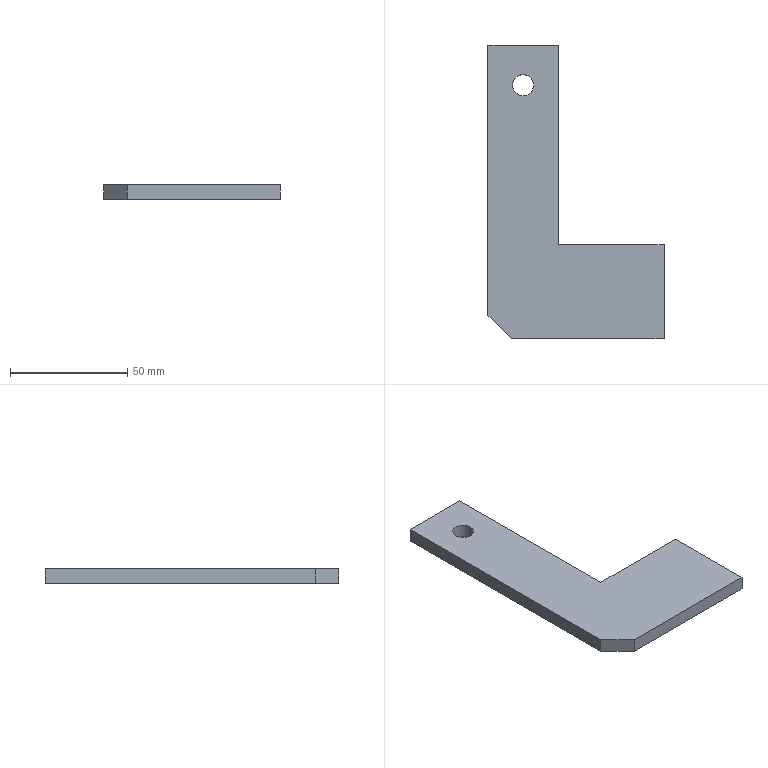Part | SolidWorks | features Chamfer 1, Extrusion 1, ICE 1 | 1 solid | 11 faces | box 75 x 125 x 6 mm | volume 32618 mm3 | plane 9 | cylinder 2 | commonest cylinder face diameters 9 x2
STEP:
#1=CARTESIAN_POINT('',(-23.022,21.378,0.));
#2=VERTEX_POINT('',#1);
#3=CARTESIAN_POINT('',(-14.022,21.378,0.));
#4=VERTEX_POINT('',#3);
#5=CARTESIAN_POINT('',(-18.522,21.378,0.));
#6=DIRECTION('',(0.,0.,1.));
#7=DIRECTION('',(-1.,0.,0.));
#8=AXIS2_PLACEMENT_3D('',#5,#6,#7);
#9=CIRCLE('',#8,4.5);
#10=EDGE_CURVE('',#2,#4,#9,.T.);
#11=ORIENTED_EDGE('',*,*,#10,.F.);
#12=CARTESIAN_POINT('',(-23.022,21.378,6.));
#13=VERTEX_POINT('',#12);
#14=CARTESIAN_POINT('',(-23.022,21.378,-0.001));
#15=DIRECTION('',(0.,0.,1.));
#16=VECTOR('',#15,1000.);
#17=LINE('',#14,#16);
#18=EDGE_CURVE('',#2,#13,#17,.T.);
#19=ORIENTED_EDGE('',*,*,#18,.T.);
#20=CARTESIAN_POINT('',(-14.022,21.378,6.));
#21=VERTEX_POINT('',#20);
#22=CARTESIAN_POINT('',(-18.522,21.378,6.));
#23=DIRECTION('',(0.,0.,1.));
#24=DIRECTION('',(1.,0.,0.));
#25=AXIS2_PLACEMENT_3D('',#22,#23,#24);
#26=CIRCLE('',#25,4.5);
#27=EDGE_CURVE('',#13,#21,#26,.T.);
#28=ORIENTED_EDGE('',*,*,#27,.T.);
#29=CARTESIAN_POINT('',(-14.022,21.378,-0.001));
#30=DIRECTION('',(0.,0.,1.));
#31=VECTOR('',#30,1000.);
#32=LINE('',#29,#31);
#33=EDGE_CURVE('',#4,#21,#32,.T.);
#34=ORIENTED_EDGE('',*,*,#33,.F.);
#35=EDGE_LOOP('',(#11,#19,#28,#34));
#36=FACE_OUTER_BOUND('',#35,.T.);
#37=CARTESIAN_POINT('',(-18.522,21.378,-0.001));
#38=DIRECTION('',(0.,0.,1.));
#39=DIRECTION('',(1.,0.,0.));
#40=AXIS2_PLACEMENT_3D('',#37,#38,#39);
#41=CYLINDRICAL_SURFACE('',#40,4.5);
#42=ADVANCED_FACE('',(#36),#41,.F.);
#43=CARTESIAN_POINT('',(-23.522,-86.622,6.));
#44=VERTEX_POINT('',#43);
#45=CARTESIAN_POINT('',(41.478,-86.622,6.));
#46=VERTEX_POINT('',#45);
#47=CARTESIAN_POINT('',(41.478,-86.622,6.));
#48=DIRECTION('',(1.,0.,0.));
#49=VECTOR('',#48,1000.);
#50=LINE('',#47,#49);
#51=EDGE_CURVE('',#44,#46,#50,.T.);
#52=ORIENTED_EDGE('',*,*,#51,.F.);
#53=CARTESIAN_POINT('',(-23.522,-86.622,0.));
#54=VERTEX_POINT('',#53);
#55=CARTESIAN_POINT('',(-23.522,-86.622,6.));
#56=DIRECTION('',(0.,0.,-1.));
#57=VECTOR('',#56,1000.);
#58=LINE('',#55,#57);
#59=EDGE_CURVE('',#44,#54,#58,.T.);
#60=ORIENTED_EDGE('',*,*,#59,.T.);
#61=CARTESIAN_POINT('',(41.478,-86.622,0.));
#62=VERTEX_POINT('',#61);
#63=CARTESIAN_POINT('',(41.478,-86.622,0.));
#64=DIRECTION('',(1.,0.,0.));
#65=VECTOR('',#64,1000.);
#66=LINE('',#63,#65);
#67=EDGE_CURVE('',#54,#62,#66,.T.);
#68=ORIENTED_EDGE('',*,*,#67,.T.);
#69=CARTESIAN_POINT('',(41.478,-86.622,6.));
#70=DIRECTION('',(0.,0.,-1.));
#71=VECTOR('',#70,1000.);
#72=LINE('',#69,#71);
#73=EDGE_CURVE('',#46,#62,#72,.T.);
#74=ORIENTED_EDGE('',*,*,#73,.F.);
#75=EDGE_LOOP('',(#52,#60,#68,#74));
#76=FACE_OUTER_BOUND('',#75,.T.);
#77=CARTESIAN_POINT('',(41.478,-86.622,6.));
#78=DIRECTION('',(0.,1.,0.));
#79=DIRECTION('',(-1.,0.,0.));
#80=AXIS2_PLACEMENT_3D('',#77,#78,#79);
#81=PLANE('',#80);
#82=ADVANCED_FACE('',(#76),#81,.F.);
#83=CARTESIAN_POINT('',(41.478,-46.622,0.));
#84=VERTEX_POINT('',#83);
#85=CARTESIAN_POINT('',(41.478,-46.622,0.));
#86=DIRECTION('',(0.,1.,0.));
#87=VECTOR('',#86,1000.);
#88=LINE('',#85,#87);
#89=EDGE_CURVE('',#62,#84,#88,.T.);
#90=ORIENTED_EDGE('',*,*,#89,.T.);
#91=CARTESIAN_POINT('',(41.478,-46.622,6.));
#92=VERTEX_POINT('',#91);
#93=CARTESIAN_POINT('',(41.478,-46.622,6.));
#94=DIRECTION('',(0.,0.,-1.));
#95=VECTOR('',#94,1000.);
#96=LINE('',#93,#95);
#97=EDGE_CURVE('',#92,#84,#96,.T.);
#98=ORIENTED_EDGE('',*,*,#97,.F.);
#99=CARTESIAN_POINT('',(41.478,-46.622,6.));
#100=DIRECTION('',(0.,1.,0.));
#101=VECTOR('',#100,1000.);
#102=LINE('',#99,#101);
#103=EDGE_CURVE('',#46,#92,#102,.T.);
#104=ORIENTED_EDGE('',*,*,#103,.F.);
#105=ORIENTED_EDGE('',*,*,#73,.T.);
#106=EDGE_LOOP('',(#90,#98,#104,#105));
#107=FACE_OUTER_BOUND('',#106,.T.);
#108=CARTESIAN_POINT('',(41.478,-46.622,6.));
#109=DIRECTION('',(-1.,0.,0.));
#110=DIRECTION('',(0.,-1.,0.));
#111=AXIS2_PLACEMENT_3D('',#108,#109,#110);
#112=PLANE('',#111);
#113=ADVANCED_FACE('',(#107),#112,.F.);
#114=CARTESIAN_POINT('',(-3.522,-46.622,0.));
#115=VERTEX_POINT('',#114);
#116=CARTESIAN_POINT('',(-3.522,-46.622,0.));
#117=DIRECTION('',(-1.,0.,0.));
#118=VECTOR('',#117,1000.);
#119=LINE('',#116,#118);
#120=EDGE_CURVE('',#84,#115,#119,.T.);
#121=ORIENTED_EDGE('',*,*,#120,.T.);
#122=CARTESIAN_POINT('',(-3.522,-46.622,6.));
#123=VERTEX_POINT('',#122);
#124=CARTESIAN_POINT('',(-3.522,-46.622,6.));
#125=DIRECTION('',(0.,0.,-1.));
#126=VECTOR('',#125,1000.);
#127=LINE('',#124,#126);
#128=EDGE_CURVE('',#123,#115,#127,.T.);
#129=ORIENTED_EDGE('',*,*,#128,.F.);
#130=CARTESIAN_POINT('',(-3.522,-46.622,6.));
#131=DIRECTION('',(-1.,0.,0.));
#132=VECTOR('',#131,1000.);
#133=LINE('',#130,#132);
#134=EDGE_CURVE('',#92,#123,#133,.T.);
#135=ORIENTED_EDGE('',*,*,#134,.F.);
#136=ORIENTED_EDGE('',*,*,#97,.T.);
#137=EDGE_LOOP('',(#121,#129,#135,#136));
#138=FACE_OUTER_BOUND('',#137,.T.);
#139=CARTESIAN_POINT('',(-3.522,-46.622,6.));
#140=DIRECTION('',(0.,-1.,0.));
#141=DIRECTION('',(0.,0.,-1.));
#142=AXIS2_PLACEMENT_3D('',#139,#140,#141);
#143=PLANE('',#142);
#144=ADVANCED_FACE('',(#138),#143,.F.);
#145=CARTESIAN_POINT('',(-3.522,38.378,0.));
#146=VERTEX_POINT('',#145);
#147=CARTESIAN_POINT('',(-3.522,38.378,0.));
#148=DIRECTION('',(0.,1.,0.));
#149=VECTOR('',#148,1000.);
#150=LINE('',#147,#149);
#151=EDGE_CURVE('',#115,#146,#150,.T.);
#152=ORIENTED_EDGE('',*,*,#151,.T.);
#153=CARTESIAN_POINT('',(-3.522,38.378,6.));
#154=VERTEX_POINT('',#153);
#155=CARTESIAN_POINT('',(-3.522,38.378,6.));
#156=DIRECTION('',(0.,0.,-1.));
#157=VECTOR('',#156,1000.);
#158=LINE('',#155,#157);
#159=EDGE_CURVE('',#154,#146,#158,.T.);
#160=ORIENTED_EDGE('',*,*,#159,.F.);
#161=CARTESIAN_POINT('',(-3.522,38.378,6.));
#162=DIRECTION('',(0.,1.,0.));
#163=VECTOR('',#162,1000.);
#164=LINE('',#161,#163);
#165=EDGE_CURVE('',#123,#154,#164,.T.);
#166=ORIENTED_EDGE('',*,*,#165,.F.);
#167=ORIENTED_EDGE('',*,*,#128,.T.);
#168=EDGE_LOOP('',(#152,#160,#166,#167));
#169=FACE_OUTER_BOUND('',#168,.T.);
#170=CARTESIAN_POINT('',(-3.522,38.378,6.));
#171=DIRECTION('',(-1.,0.,0.));
#172=DIRECTION('',(0.,-1.,0.));
#173=AXIS2_PLACEMENT_3D('',#170,#171,#172);
#174=PLANE('',#173);
#175=ADVANCED_FACE('',(#169),#174,.F.);
#176=CARTESIAN_POINT('',(-33.522,38.378,0.));
#177=VERTEX_POINT('',#176);
#178=CARTESIAN_POINT('',(-33.522,38.378,0.));
#179=DIRECTION('',(-1.,0.,0.));
#180=VECTOR('',#179,1000.);
#181=LINE('',#178,#180);
#182=EDGE_CURVE('',#146,#177,#181,.T.);
#183=ORIENTED_EDGE('',*,*,#182,.T.);
#184=CARTESIAN_POINT('',(-33.522,38.378,6.));
#185=VERTEX_POINT('',#184);
#186=CARTESIAN_POINT('',(-33.522,38.378,6.));
#187=DIRECTION('',(0.,0.,-1.));
#188=VECTOR('',#187,1000.);
#189=LINE('',#186,#188);
#190=EDGE_CURVE('',#185,#177,#189,.T.);
#191=ORIENTED_EDGE('',*,*,#190,.F.);
#192=CARTESIAN_POINT('',(-33.522,38.378,6.));
#193=DIRECTION('',(-1.,0.,0.));
#194=VECTOR('',#193,1000.);
#195=LINE('',#192,#194);
#196=EDGE_CURVE('',#154,#185,#195,.T.);
#197=ORIENTED_EDGE('',*,*,#196,.F.);
#198=ORIENTED_EDGE('',*,*,#159,.T.);
#199=EDGE_LOOP('',(#183,#191,#197,#198));
#200=FACE_OUTER_BOUND('',#199,.T.);
#201=CARTESIAN_POINT('',(-33.522,38.378,6.));
#202=DIRECTION('',(0.,-1.,0.));
#203=DIRECTION('',(0.,0.,-1.));
#204=AXIS2_PLACEMENT_3D('',#201,#202,#203);
#205=PLANE('',#204);
#206=ADVANCED_FACE('',(#200),#205,.F.);
#207=CARTESIAN_POINT('',(-33.522,-76.622,0.));
#208=VERTEX_POINT('',#207);
#209=CARTESIAN_POINT('',(-33.522,-86.622,0.));
#210=DIRECTION('',(0.,-1.,0.));
#211=VECTOR('',#210,1000.);
#212=LINE('',#209,#211);
#213=EDGE_CURVE('',#177,#208,#212,.T.);
#214=ORIENTED_EDGE('',*,*,#213,.T.);
#215=CARTESIAN_POINT('',(-33.522,-76.622,6.));
#216=VERTEX_POINT('',#215);
#217=CARTESIAN_POINT('',(-33.522,-76.622,6.));
#218=DIRECTION('',(0.,0.,1.));
#219=VECTOR('',#218,1000.);
#220=LINE('',#217,#219);
#221=EDGE_CURVE('',#208,#216,#220,.T.);
#222=ORIENTED_EDGE('',*,*,#221,.T.);
#223=CARTESIAN_POINT('',(-33.522,-86.622,6.));
#224=DIRECTION('',(0.,-1.,0.));
#225=VECTOR('',#224,1000.);
#226=LINE('',#223,#225);
#227=EDGE_CURVE('',#185,#216,#226,.T.);
#228=ORIENTED_EDGE('',*,*,#227,.F.);
#229=ORIENTED_EDGE('',*,*,#190,.T.);
#230=EDGE_LOOP('',(#214,#222,#228,#229));
#231=FACE_OUTER_BOUND('',#230,.T.);
#232=CARTESIAN_POINT('',(-33.522,-86.622,6.));
#233=DIRECTION('',(1.,0.,0.));
#234=DIRECTION('',(0.,0.,-1.));
#235=AXIS2_PLACEMENT_3D('',#232,#233,#234);
#236=PLANE('',#235);
#237=ADVANCED_FACE('',(#231),#236,.F.);
#238=CARTESIAN_POINT('',(-18.522,21.378,6.));
#239=DIRECTION('',(0.,0.,1.));
#240=DIRECTION('',(1.,0.,0.));
#241=AXIS2_PLACEMENT_3D('',#238,#239,#240);
#242=CIRCLE('',#241,4.5);
#243=EDGE_CURVE('',#21,#13,#242,.T.);
#244=ORIENTED_EDGE('',*,*,#243,.F.);
#245=ORIENTED_EDGE('',*,*,#27,.F.);
#246=EDGE_LOOP('',(#244,#245));
#247=FACE_BOUND('',#246,.T.);
#248=ORIENTED_EDGE('',*,*,#227,.T.);
#249=CARTESIAN_POINT('',(-23.522,-86.622,6.));
#250=DIRECTION('',(0.7071,-0.7071,0.));
#251=VECTOR('',#250,1000.);
#252=LINE('',#249,#251);
#253=EDGE_CURVE('',#216,#44,#252,.T.);
#254=ORIENTED_EDGE('',*,*,#253,.T.);
#255=ORIENTED_EDGE('',*,*,#51,.T.);
#256=ORIENTED_EDGE('',*,*,#103,.T.);
#257=ORIENTED_EDGE('',*,*,#134,.T.);
#258=ORIENTED_EDGE('',*,*,#165,.T.);
#259=ORIENTED_EDGE('',*,*,#196,.T.);
#260=EDGE_LOOP('',(#248,#254,#255,#256,#257,#258,#259));
#261=FACE_OUTER_BOUND('',#260,.T.);
#262=CARTESIAN_POINT('',(0.,0.,6.));
#263=DIRECTION('',(0.,0.,-1.));
#264=DIRECTION('',(-1.,0.,0.));
#265=AXIS2_PLACEMENT_3D('',#262,#263,#264);
#266=PLANE('',#265);
#267=ADVANCED_FACE('',(#247,#261),#266,.F.);
#268=CARTESIAN_POINT('',(-18.522,21.378,0.));
#269=DIRECTION('',(0.,0.,1.));
#270=DIRECTION('',(-1.,0.,0.));
#271=AXIS2_PLACEMENT_3D('',#268,#269,#270);
#272=CIRCLE('',#271,4.5);
#273=EDGE_CURVE('',#4,#2,#272,.T.);
#274=ORIENTED_EDGE('',*,*,#273,.T.);
#275=ORIENTED_EDGE('',*,*,#10,.T.);
#276=EDGE_LOOP('',(#274,#275));
#277=FACE_BOUND('',#276,.T.);
#278=ORIENTED_EDGE('',*,*,#67,.F.);
#279=CARTESIAN_POINT('',(-55.072,-55.072,0.));
#280=DIRECTION('',(-0.7071,0.7071,0.));
#281=VECTOR('',#280,1000.);
#282=LINE('',#279,#281);
#283=EDGE_CURVE('',#54,#208,#282,.T.);
#284=ORIENTED_EDGE('',*,*,#283,.T.);
#285=ORIENTED_EDGE('',*,*,#213,.F.);
#286=ORIENTED_EDGE('',*,*,#182,.F.);
#287=ORIENTED_EDGE('',*,*,#151,.F.);
#288=ORIENTED_EDGE('',*,*,#120,.F.);
#289=ORIENTED_EDGE('',*,*,#89,.F.);
#290=EDGE_LOOP('',(#278,#284,#285,#286,#287,#288,#289));
#291=FACE_OUTER_BOUND('',#290,.T.);
#292=CARTESIAN_POINT('',(0.,0.,0.));
#293=DIRECTION('',(0.,0.,-1.));
#294=DIRECTION('',(-1.,0.,0.));
#295=AXIS2_PLACEMENT_3D('',#292,#293,#294);
#296=PLANE('',#295);
#297=ADVANCED_FACE('',(#277,#291),#296,.T.);
#298=ORIENTED_EDGE('',*,*,#18,.F.);
#299=ORIENTED_EDGE('',*,*,#273,.F.);
#300=ORIENTED_EDGE('',*,*,#33,.T.);
#301=ORIENTED_EDGE('',*,*,#243,.T.);
#302=EDGE_LOOP('',(#298,#299,#300,#301));
#303=FACE_OUTER_BOUND('',#302,.T.);
#304=CARTESIAN_POINT('',(-18.522,21.378,-0.001));
#305=DIRECTION('',(0.,0.,1.));
#306=DIRECTION('',(1.,0.,0.));
#307=AXIS2_PLACEMENT_3D('',#304,#305,#306);
#308=CYLINDRICAL_SURFACE('',#307,4.5);
#309=ADVANCED_FACE('',(#303),#308,.F.);
#310=ORIENTED_EDGE('',*,*,#253,.F.);
#311=ORIENTED_EDGE('',*,*,#221,.F.);
#312=ORIENTED_EDGE('',*,*,#283,.F.);
#313=ORIENTED_EDGE('',*,*,#59,.F.);
#314=EDGE_LOOP('',(#310,#311,#312,#313));
#315=FACE_OUTER_BOUND('',#314,.T.);
#316=CARTESIAN_POINT('',(-23.522,-86.622,6.));
#317=DIRECTION('',(0.7071,0.7071,0.));
#318=DIRECTION('',(0.,0.,-1.));
#319=AXIS2_PLACEMENT_3D('',#316,#317,#318);
#320=PLANE('',#319);
#321=ADVANCED_FACE('',(#315),#320,.F.);
#322=CLOSED_SHELL('',(#42,#82,#113,#144,#175,#206,#237,#267,#297,#309,#321));
#323=MANIFOLD_SOLID_BREP('',#322);
#324=CARTESIAN_POINT('',(0.,0.,0.));
#325=DIRECTION('',(0.,0.,1.));
#326=DIRECTION('',(1.,0.,0.));
#327=AXIS2_PLACEMENT_3D('',#324,#325,#326);
#328=(LENGTH_UNIT()NAMED_UNIT(*)SI_UNIT(.MILLI.,.METRE.));
#329=UNCERTAINTY_MEASURE_WITH_UNIT(LENGTH_MEASURE(0.00001),#328,'','');
#330=(NAMED_UNIT(*)PLANE_ANGLE_UNIT()SI_UNIT($,.RADIAN.));
#331=(NAMED_UNIT(*)SI_UNIT($,.STERADIAN.)SOLID_ANGLE_UNIT());
#332=(GEOMETRIC_REPRESENTATION_CONTEXT(3)GLOBAL_UNCERTAINTY_ASSIGNED_CONTEXT((#329))GLOBAL_UNIT_ASSIGNED_CONTEXT((#328,#330,#331))REPRESENTATION_CONTEXT('',''));
#333=ADVANCED_BREP_SHAPE_REPRESENTATION('',(#323,#327),#332);